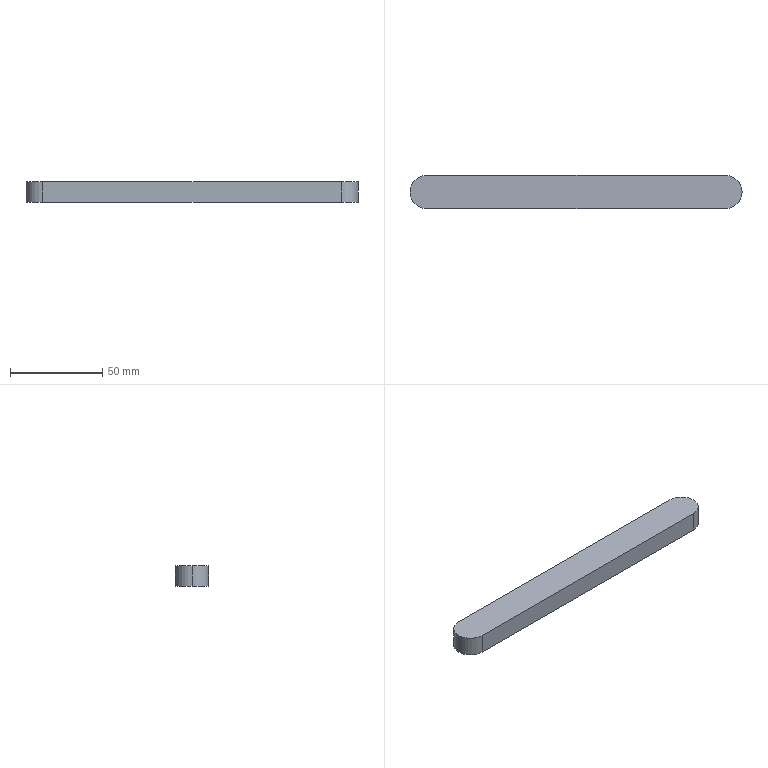Part | SolidWorks | features Extrusion 1, Fillet 1 | 1 solid | 8 faces | box 180 x 18 x 11 mm | volume 34875 mm3 | plane 4 | cylinder 4 | commonest cylinder face diameters 18 x4
STEP:
#1=CARTESIAN_POINT('',(81.,9.,11.));
#2=VERTEX_POINT('',#1);
#3=CARTESIAN_POINT('',(-81.,9.,11.));
#4=VERTEX_POINT('',#3);
#5=CARTESIAN_POINT('',(-90.,9.,11.));
#6=DIRECTION('',(-1.,0.,0.));
#7=VECTOR('',#6,1000.);
#8=LINE('',#5,#7);
#9=EDGE_CURVE('',#2,#4,#8,.T.);
#10=ORIENTED_EDGE('',*,*,#9,.F.);
#11=CARTESIAN_POINT('',(81.,9.,0.));
#12=VERTEX_POINT('',#11);
#13=CARTESIAN_POINT('',(81.,9.,11.));
#14=DIRECTION('',(0.,0.,-1.));
#15=VECTOR('',#14,1000.);
#16=LINE('',#13,#15);
#17=EDGE_CURVE('',#2,#12,#16,.T.);
#18=ORIENTED_EDGE('',*,*,#17,.T.);
#19=CARTESIAN_POINT('',(-81.,9.,0.));
#20=VERTEX_POINT('',#19);
#21=CARTESIAN_POINT('',(-90.,9.,0.));
#22=DIRECTION('',(-1.,0.,0.));
#23=VECTOR('',#22,1000.);
#24=LINE('',#21,#23);
#25=EDGE_CURVE('',#12,#20,#24,.T.);
#26=ORIENTED_EDGE('',*,*,#25,.T.);
#27=CARTESIAN_POINT('',(-81.,9.,11.));
#28=DIRECTION('',(0.,0.,1.));
#29=VECTOR('',#28,1000.);
#30=LINE('',#27,#29);
#31=EDGE_CURVE('',#20,#4,#30,.T.);
#32=ORIENTED_EDGE('',*,*,#31,.T.);
#33=EDGE_LOOP('',(#10,#18,#26,#32));
#34=FACE_OUTER_BOUND('',#33,.T.);
#35=CARTESIAN_POINT('',(-90.,9.,11.));
#36=DIRECTION('',(0.,-1.,0.));
#37=DIRECTION('',(0.,0.,-1.));
#38=AXIS2_PLACEMENT_3D('',#35,#36,#37);
#39=PLANE('',#38);
#40=ADVANCED_FACE('',(#34),#39,.F.);
#41=CARTESIAN_POINT('',(-81.,-9.,0.));
#42=VERTEX_POINT('',#41);
#43=CARTESIAN_POINT('',(81.,-9.,0.));
#44=VERTEX_POINT('',#43);
#45=CARTESIAN_POINT('',(-90.,-9.,0.));
#46=DIRECTION('',(1.,0.,0.));
#47=VECTOR('',#46,1000.);
#48=LINE('',#45,#47);
#49=EDGE_CURVE('',#42,#44,#48,.T.);
#50=ORIENTED_EDGE('',*,*,#49,.T.);
#51=CARTESIAN_POINT('',(81.,-9.,11.));
#52=VERTEX_POINT('',#51);
#53=CARTESIAN_POINT('',(81.,-9.,11.));
#54=DIRECTION('',(0.,0.,1.));
#55=VECTOR('',#54,1000.);
#56=LINE('',#53,#55);
#57=EDGE_CURVE('',#44,#52,#56,.T.);
#58=ORIENTED_EDGE('',*,*,#57,.T.);
#59=CARTESIAN_POINT('',(-81.,-9.,11.));
#60=VERTEX_POINT('',#59);
#61=CARTESIAN_POINT('',(-90.,-9.,11.));
#62=DIRECTION('',(1.,0.,0.));
#63=VECTOR('',#62,1000.);
#64=LINE('',#61,#63);
#65=EDGE_CURVE('',#60,#52,#64,.T.);
#66=ORIENTED_EDGE('',*,*,#65,.F.);
#67=CARTESIAN_POINT('',(-81.,-9.,11.));
#68=DIRECTION('',(0.,0.,-1.));
#69=VECTOR('',#68,1000.);
#70=LINE('',#67,#69);
#71=EDGE_CURVE('',#60,#42,#70,.T.);
#72=ORIENTED_EDGE('',*,*,#71,.T.);
#73=EDGE_LOOP('',(#50,#58,#66,#72));
#74=FACE_OUTER_BOUND('',#73,.T.);
#75=CARTESIAN_POINT('',(-90.,-9.,11.));
#76=DIRECTION('',(0.,1.,0.));
#77=DIRECTION('',(0.,0.,1.));
#78=AXIS2_PLACEMENT_3D('',#75,#76,#77);
#79=PLANE('',#78);
#80=ADVANCED_FACE('',(#74),#79,.F.);
#81=CARTESIAN_POINT('',(90.,0.,11.));
#82=VERTEX_POINT('',#81);
#83=CARTESIAN_POINT('',(81.,0.,11.));
#84=DIRECTION('',(0.,0.,1.));
#85=DIRECTION('',(1.,0.,0.));
#86=AXIS2_PLACEMENT_3D('',#83,#84,#85);
#87=CIRCLE('',#86,9.);
#88=EDGE_CURVE('',#52,#82,#87,.T.);
#89=ORIENTED_EDGE('',*,*,#88,.T.);
#90=CARTESIAN_POINT('',(81.,0.,11.));
#91=DIRECTION('',(0.,0.,1.));
#92=DIRECTION('',(1.,0.,0.));
#93=AXIS2_PLACEMENT_3D('',#90,#91,#92);
#94=CIRCLE('',#93,9.);
#95=EDGE_CURVE('',#82,#2,#94,.T.);
#96=ORIENTED_EDGE('',*,*,#95,.T.);
#97=ORIENTED_EDGE('',*,*,#9,.T.);
#98=CARTESIAN_POINT('',(-90.,0.,11.));
#99=VERTEX_POINT('',#98);
#100=CARTESIAN_POINT('',(-81.,0.,11.));
#101=DIRECTION('',(0.,0.,1.));
#102=DIRECTION('',(1.,0.,0.));
#103=AXIS2_PLACEMENT_3D('',#100,#101,#102);
#104=CIRCLE('',#103,9.);
#105=EDGE_CURVE('',#4,#99,#104,.T.);
#106=ORIENTED_EDGE('',*,*,#105,.T.);
#107=CARTESIAN_POINT('',(-81.,0.,11.));
#108=DIRECTION('',(0.,0.,1.));
#109=DIRECTION('',(1.,0.,0.));
#110=AXIS2_PLACEMENT_3D('',#107,#108,#109);
#111=CIRCLE('',#110,9.);
#112=EDGE_CURVE('',#99,#60,#111,.T.);
#113=ORIENTED_EDGE('',*,*,#112,.T.);
#114=ORIENTED_EDGE('',*,*,#65,.T.);
#115=EDGE_LOOP('',(#89,#96,#97,#106,#113,#114));
#116=FACE_OUTER_BOUND('',#115,.T.);
#117=CARTESIAN_POINT('',(0.,0.,11.));
#118=DIRECTION('',(0.,0.,1.));
#119=DIRECTION('',(1.,0.,0.));
#120=AXIS2_PLACEMENT_3D('',#117,#118,#119);
#121=PLANE('',#120);
#122=ADVANCED_FACE('',(#116),#121,.T.);
#123=ORIENTED_EDGE('',*,*,#25,.F.);
#124=CARTESIAN_POINT('',(90.,0.,0.));
#125=VERTEX_POINT('',#124);
#126=CARTESIAN_POINT('',(81.,0.,0.));
#127=DIRECTION('',(0.,0.,-1.));
#128=DIRECTION('',(1.,0.,0.));
#129=AXIS2_PLACEMENT_3D('',#126,#127,#128);
#130=CIRCLE('',#129,9.);
#131=EDGE_CURVE('',#12,#125,#130,.T.);
#132=ORIENTED_EDGE('',*,*,#131,.T.);
#133=CARTESIAN_POINT('',(81.,0.,0.));
#134=DIRECTION('',(0.,0.,-1.));
#135=DIRECTION('',(1.,0.,0.));
#136=AXIS2_PLACEMENT_3D('',#133,#134,#135);
#137=CIRCLE('',#136,9.);
#138=EDGE_CURVE('',#125,#44,#137,.T.);
#139=ORIENTED_EDGE('',*,*,#138,.T.);
#140=ORIENTED_EDGE('',*,*,#49,.F.);
#141=CARTESIAN_POINT('',(-90.,0.,0.));
#142=VERTEX_POINT('',#141);
#143=CARTESIAN_POINT('',(-81.,0.,0.));
#144=DIRECTION('',(0.,0.,-1.));
#145=DIRECTION('',(1.,0.,0.));
#146=AXIS2_PLACEMENT_3D('',#143,#144,#145);
#147=CIRCLE('',#146,9.);
#148=EDGE_CURVE('',#42,#142,#147,.T.);
#149=ORIENTED_EDGE('',*,*,#148,.T.);
#150=CARTESIAN_POINT('',(-81.,0.,0.));
#151=DIRECTION('',(0.,0.,-1.));
#152=DIRECTION('',(1.,0.,0.));
#153=AXIS2_PLACEMENT_3D('',#150,#151,#152);
#154=CIRCLE('',#153,9.);
#155=EDGE_CURVE('',#142,#20,#154,.T.);
#156=ORIENTED_EDGE('',*,*,#155,.T.);
#157=EDGE_LOOP('',(#123,#132,#139,#140,#149,#156));
#158=FACE_OUTER_BOUND('',#157,.T.);
#159=CARTESIAN_POINT('',(0.,0.,0.));
#160=DIRECTION('',(0.,0.,1.));
#161=DIRECTION('',(1.,0.,0.));
#162=AXIS2_PLACEMENT_3D('',#159,#160,#161);
#163=PLANE('',#162);
#164=ADVANCED_FACE('',(#158),#163,.F.);
#165=CARTESIAN_POINT('',(90.,0.,11.));
#166=DIRECTION('',(0.,0.,-1.));
#167=VECTOR('',#166,1000.);
#168=LINE('',#165,#167);
#169=EDGE_CURVE('',#82,#125,#168,.T.);
#170=ORIENTED_EDGE('',*,*,#169,.F.);
#171=ORIENTED_EDGE('',*,*,#88,.F.);
#172=ORIENTED_EDGE('',*,*,#57,.F.);
#173=ORIENTED_EDGE('',*,*,#138,.F.);
#174=EDGE_LOOP('',(#170,#171,#172,#173));
#175=FACE_OUTER_BOUND('',#174,.T.);
#176=CARTESIAN_POINT('',(81.,0.,11.));
#177=DIRECTION('',(0.,0.,-1.));
#178=DIRECTION('',(-1.,0.,0.));
#179=AXIS2_PLACEMENT_3D('',#176,#177,#178);
#180=CYLINDRICAL_SURFACE('',#179,9.);
#181=ADVANCED_FACE('',(#175),#180,.T.);
#182=ORIENTED_EDGE('',*,*,#95,.F.);
#183=ORIENTED_EDGE('',*,*,#169,.T.);
#184=ORIENTED_EDGE('',*,*,#131,.F.);
#185=ORIENTED_EDGE('',*,*,#17,.F.);
#186=EDGE_LOOP('',(#182,#183,#184,#185));
#187=FACE_OUTER_BOUND('',#186,.T.);
#188=CARTESIAN_POINT('',(81.,0.,11.));
#189=DIRECTION('',(0.,0.,-1.));
#190=DIRECTION('',(-1.,0.,0.));
#191=AXIS2_PLACEMENT_3D('',#188,#189,#190);
#192=CYLINDRICAL_SURFACE('',#191,9.);
#193=ADVANCED_FACE('',(#187),#192,.T.);
#194=CARTESIAN_POINT('',(-90.,0.,11.));
#195=DIRECTION('',(0.,0.,-1.));
#196=VECTOR('',#195,1000.);
#197=LINE('',#194,#196);
#198=EDGE_CURVE('',#99,#142,#197,.T.);
#199=ORIENTED_EDGE('',*,*,#198,.F.);
#200=ORIENTED_EDGE('',*,*,#105,.F.);
#201=ORIENTED_EDGE('',*,*,#31,.F.);
#202=ORIENTED_EDGE('',*,*,#155,.F.);
#203=EDGE_LOOP('',(#199,#200,#201,#202));
#204=FACE_OUTER_BOUND('',#203,.T.);
#205=CARTESIAN_POINT('',(-81.,0.,11.));
#206=DIRECTION('',(0.,0.,-1.));
#207=DIRECTION('',(-1.,0.,0.));
#208=AXIS2_PLACEMENT_3D('',#205,#206,#207);
#209=CYLINDRICAL_SURFACE('',#208,9.);
#210=ADVANCED_FACE('',(#204),#209,.T.);
#211=ORIENTED_EDGE('',*,*,#112,.F.);
#212=ORIENTED_EDGE('',*,*,#198,.T.);
#213=ORIENTED_EDGE('',*,*,#148,.F.);
#214=ORIENTED_EDGE('',*,*,#71,.F.);
#215=EDGE_LOOP('',(#211,#212,#213,#214));
#216=FACE_OUTER_BOUND('',#215,.T.);
#217=CARTESIAN_POINT('',(-81.,0.,11.));
#218=DIRECTION('',(0.,0.,-1.));
#219=DIRECTION('',(-1.,0.,0.));
#220=AXIS2_PLACEMENT_3D('',#217,#218,#219);
#221=CYLINDRICAL_SURFACE('',#220,9.);
#222=ADVANCED_FACE('',(#216),#221,.T.);
#223=CLOSED_SHELL('',(#40,#80,#122,#164,#181,#193,#210,#222));
#224=MANIFOLD_SOLID_BREP('',#223);
#225=CARTESIAN_POINT('',(0.,0.,0.));
#226=DIRECTION('',(0.,0.,1.));
#227=DIRECTION('',(1.,0.,0.));
#228=AXIS2_PLACEMENT_3D('',#225,#226,#227);
#229=(LENGTH_UNIT()NAMED_UNIT(*)SI_UNIT(.MILLI.,.METRE.));
#230=UNCERTAINTY_MEASURE_WITH_UNIT(LENGTH_MEASURE(0.00001),#229,'','');
#231=(NAMED_UNIT(*)PLANE_ANGLE_UNIT()SI_UNIT($,.RADIAN.));
#232=(NAMED_UNIT(*)SI_UNIT($,.STERADIAN.)SOLID_ANGLE_UNIT());
#233=(GEOMETRIC_REPRESENTATION_CONTEXT(3)GLOBAL_UNCERTAINTY_ASSIGNED_CONTEXT((#230))GLOBAL_UNIT_ASSIGNED_CONTEXT((#229,#231,#232))REPRESENTATION_CONTEXT('',''));
#234=ADVANCED_BREP_SHAPE_REPRESENTATION('',(#224,#228),#233);